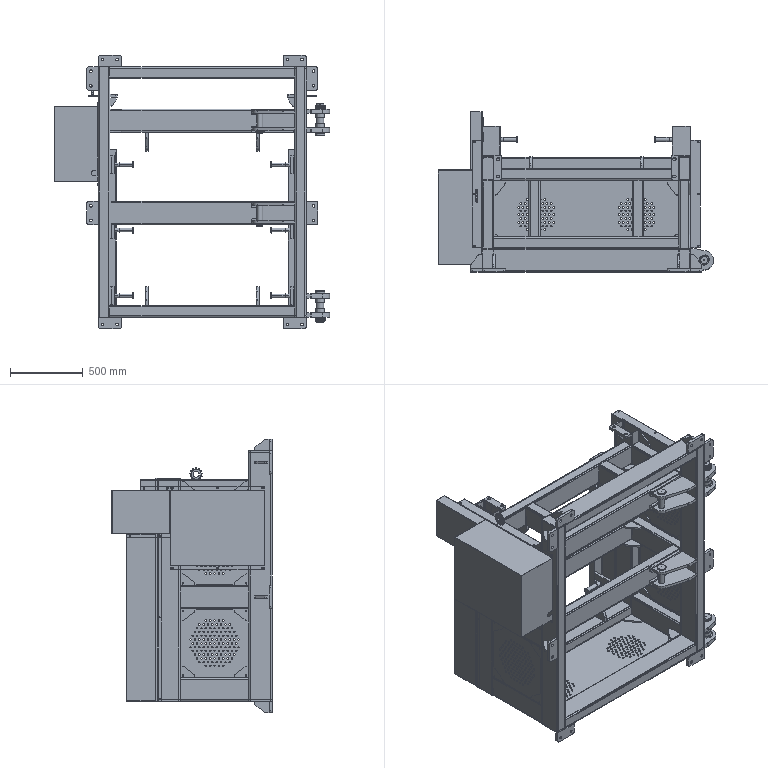Part | SolidWorks | 267 solids | 12348 faces | volume 86480189 mm3 | plane 8058 | cylinder 3420 | cone 770 | torus 92 | spline 8 | commonest cylinder face diameters 5.96 x480 7 x384 18.08 x360 83.184 x240 10 x230 20 x156